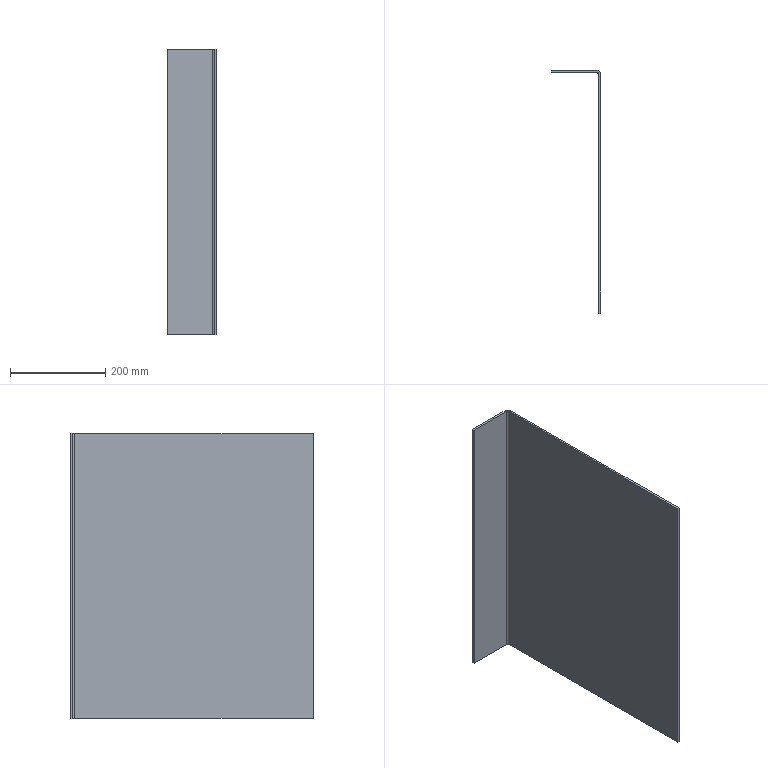Part | STEP file | 03-Side middle pedal | 1 solid | 14 faces | box 104 x 510 x 600 mm | volume 1457819 mm3 | plane 12 | cylinder 2 | commonest cylinder face diameters 8 x1 16 x1
STEP:
#1=CARTESIAN_POINT('',(0.,0.,0.));
#2=DIRECTION('',(0.,0.,1.));
#3=DIRECTION('',(1.,0.,0.));
#4=AXIS2_PLACEMENT_3D('',#1,#2,#3);
#5=CARTESIAN_POINT('',(104.,-8.,600.));
#6=VERTEX_POINT('',#5);
#7=CARTESIAN_POINT('',(100.,-8.,600.));
#8=VERTEX_POINT('',#7);
#9=CARTESIAN_POINT('',(104.,-8.,600.));
#10=DIRECTION('',(-1.,0.,0.));
#11=VECTOR('',#10,1.);
#12=LINE('',#9,#11);
#13=CARTESIAN_POINT('',(104.,-8.,600.));
#14=DIRECTION('',(0.,0.,1.));
#15=DIRECTION('',(1.,0.,0.));
#16=AXIS2_PLACEMENT_3D('',#13,#14,#15);
#17=PLANE('',#16);
#18=CARTESIAN_POINT('',(0.,0.));
#19=DIRECTION('',(-1.,0.));
#20=VECTOR('',#19,1.);
#21=LINE('',#18,#20);
#22=(GEOMETRIC_REPRESENTATION_CONTEXT(2)PARAMETRIC_REPRESENTATION_CONTEXT()REPRESENTATION_CONTEXT('',''));
#23=DEFINITIONAL_REPRESENTATION('',(#21),#22);
#24=PCURVE('',#17,#23);
#25=CARTESIAN_POINT('',(96.,-4.,600.));
#26=DIRECTION('',(0.,0.,1.));
#27=DIRECTION('',(1.,0.,0.));
#28=AXIS2_PLACEMENT_3D('',#25,#26,#27);
#29=PLANE('',#28);
#30=CARTESIAN_POINT('',(8.,-4.));
#31=DIRECTION('',(-1.,0.));
#32=VECTOR('',#31,1.);
#33=LINE('',#30,#32);
#34=(GEOMETRIC_REPRESENTATION_CONTEXT(2)PARAMETRIC_REPRESENTATION_CONTEXT()REPRESENTATION_CONTEXT('',''));
#35=DEFINITIONAL_REPRESENTATION('',(#33),#34);
#36=PCURVE('',#29,#35);
#37=SURFACE_CURVE('',#12,(#24,#36),.PCURVE_S1.);
#38=EDGE_CURVE('',#6,#8,#37,.T.);
#39=ORIENTED_EDGE('',*,*,#38,.F.);
#40=CARTESIAN_POINT('',(96.,0.,600.));
#41=VERTEX_POINT('',#40);
#42=CARTESIAN_POINT('',(96.,-8.,600.));
#43=DIRECTION('',(0.,0.,-1.));
#44=DIRECTION('',(1.,0.,0.));
#45=AXIS2_PLACEMENT_3D('',#42,#43,#44);
#46=CIRCLE('',#45,8.);
#47=CARTESIAN_POINT('',(0.,0.));
#48=CARTESIAN_POINT('',(0.,-13.856));
#49=CARTESIAN_POINT('',(-12.,-6.928));
#50=CARTESIAN_POINT('',(-24.,0.));
#51=CARTESIAN_POINT('',(-12.,6.928));
#52=CARTESIAN_POINT('',(0.,13.856));
#53=CARTESIAN_POINT('',(0.,0.));
#54=(BOUNDED_CURVE()B_SPLINE_CURVE(2,(#47,#48,#49,#50,#51,#52,#53),.UNSPECIFIED.,.T.,.F.)B_SPLINE_CURVE_WITH_KNOTS((1,2,2,2,2,1),(-2.094,0.,2.094,4.189,6.283,8.378),.UNSPECIFIED.)CURVE()GEOMETRIC_REPRESENTATION_ITEM()RATIONAL_B_SPLINE_CURVE((1.,0.5,1.,0.5,1.,0.5,1.))REPRESENTATION_ITEM(''));
#55=(GEOMETRIC_REPRESENTATION_CONTEXT(2)PARAMETRIC_REPRESENTATION_CONTEXT()REPRESENTATION_CONTEXT('',''));
#56=DEFINITIONAL_REPRESENTATION('',(#54),#55);
#57=PCURVE('',#17,#56);
#58=CARTESIAN_POINT('',(96.,-8.,600.));
#59=DIRECTION('',(0.,0.,-1.));
#60=DIRECTION('',(-1.,0.,0.));
#61=AXIS2_PLACEMENT_3D('',#58,#59,#60);
#62=CYLINDRICAL_SURFACE('',#61,8.);
#63=CARTESIAN_POINT('',(-3.142,0.));
#64=DIRECTION('',(1.,0.));
#65=VECTOR('',#64,1.);
#66=LINE('',#63,#65);
#67=(GEOMETRIC_REPRESENTATION_CONTEXT(2)PARAMETRIC_REPRESENTATION_CONTEXT()REPRESENTATION_CONTEXT('',''));
#68=DEFINITIONAL_REPRESENTATION('',(#66),#67);
#69=PCURVE('',#62,#68);
#70=SURFACE_CURVE('',#46,(#57,#69),.PCURVE_S1.);
#71=EDGE_CURVE('',#41,#6,#70,.T.);
#72=ORIENTED_EDGE('',*,*,#71,.F.);
#73=CARTESIAN_POINT('',(96.,-4.,600.));
#74=VERTEX_POINT('',#73);
#75=CARTESIAN_POINT('',(96.,-4.,600.));
#76=DIRECTION('',(0.,1.,0.));
#77=VECTOR('',#76,1.);
#78=LINE('',#75,#77);
#79=CARTESIAN_POINT('',(-8.,4.));
#80=DIRECTION('',(0.,1.));
#81=VECTOR('',#80,1.);
#82=LINE('',#79,#81);
#83=(GEOMETRIC_REPRESENTATION_CONTEXT(2)PARAMETRIC_REPRESENTATION_CONTEXT()REPRESENTATION_CONTEXT('',''));
#84=DEFINITIONAL_REPRESENTATION('',(#82),#83);
#85=PCURVE('',#17,#84);
#86=CARTESIAN_POINT('',(96.,-8.,600.));
#87=DIRECTION('',(0.,0.,1.));
#88=DIRECTION('',(1.,0.,0.));
#89=AXIS2_PLACEMENT_3D('',#86,#87,#88);
#90=PLANE('',#89);
#91=CARTESIAN_POINT('',(0.,4.));
#92=DIRECTION('',(0.,1.));
#93=VECTOR('',#92,1.);
#94=LINE('',#91,#93);
#95=(GEOMETRIC_REPRESENTATION_CONTEXT(2)PARAMETRIC_REPRESENTATION_CONTEXT()REPRESENTATION_CONTEXT('',''));
#96=DEFINITIONAL_REPRESENTATION('',(#94),#95);
#97=PCURVE('',#90,#96);
#98=SURFACE_CURVE('',#78,(#85,#97),.PCURVE_S1.);
#99=EDGE_CURVE('',#74,#41,#98,.T.);
#100=ORIENTED_EDGE('',*,*,#99,.F.);
#101=CARTESIAN_POINT('',(96.,-8.,600.));
#102=DIRECTION('',(0.,0.,-1.));
#103=DIRECTION('',(1.,0.,0.));
#104=AXIS2_PLACEMENT_3D('',#101,#102,#103);
#105=CIRCLE('',#104,4.);
#106=CARTESIAN_POINT('',(-4.,0.));
#107=CARTESIAN_POINT('',(-4.,-6.928));
#108=CARTESIAN_POINT('',(-10.,-3.464));
#109=CARTESIAN_POINT('',(-16.,0.));
#110=CARTESIAN_POINT('',(-10.,3.464));
#111=CARTESIAN_POINT('',(-4.,6.928));
#112=CARTESIAN_POINT('',(-4.,0.));
#113=(BOUNDED_CURVE()B_SPLINE_CURVE(2,(#106,#107,#108,#109,#110,#111,#112),.UNSPECIFIED.,.T.,.F.)B_SPLINE_CURVE_WITH_KNOTS((1,2,2,2,2,1),(-2.094,0.,2.094,4.189,6.283,8.378),.UNSPECIFIED.)CURVE()GEOMETRIC_REPRESENTATION_ITEM()RATIONAL_B_SPLINE_CURVE((1.,0.5,1.,0.5,1.,0.5,1.))REPRESENTATION_ITEM(''));
#114=(GEOMETRIC_REPRESENTATION_CONTEXT(2)PARAMETRIC_REPRESENTATION_CONTEXT()REPRESENTATION_CONTEXT('',''));
#115=DEFINITIONAL_REPRESENTATION('',(#113),#114);
#116=PCURVE('',#17,#115);
#117=CARTESIAN_POINT('',(96.,-8.,600.));
#118=DIRECTION('',(0.,0.,-1.));
#119=DIRECTION('',(-1.,0.,0.));
#120=AXIS2_PLACEMENT_3D('',#117,#118,#119);
#121=CYLINDRICAL_SURFACE('',#120,4.);
#122=CARTESIAN_POINT('',(-3.142,0.));
#123=DIRECTION('',(1.,0.));
#124=VECTOR('',#123,1.);
#125=LINE('',#122,#124);
#126=(GEOMETRIC_REPRESENTATION_CONTEXT(2)PARAMETRIC_REPRESENTATION_CONTEXT()REPRESENTATION_CONTEXT('',''));
#127=DEFINITIONAL_REPRESENTATION('',(#125),#126);
#128=PCURVE('',#121,#127);
#129=SURFACE_CURVE('',#105,(#116,#128),.PCURVE_S1.);
#130=EDGE_CURVE('',#74,#8,#129,.T.);
#131=ORIENTED_EDGE('',*,*,#130,.T.);
#132=EDGE_LOOP('',(#39,#72,#100,#131));
#133=FACE_BOUND('',#132,.T.);
#134=ADVANCED_FACE('',(#133),#17,.T.);
#135=CARTESIAN_POINT('',(104.,-510.,600.));
#136=VERTEX_POINT('',#135);
#137=CARTESIAN_POINT('',(104.,0.,600.));
#138=DIRECTION('',(0.,-1.,0.));
#139=VECTOR('',#138,1.);
#140=LINE('',#137,#139);
#141=CARTESIAN_POINT('',(8.,4.));
#142=DIRECTION('',(0.,-1.));
#143=VECTOR('',#142,1.);
#144=LINE('',#141,#143);
#145=(GEOMETRIC_REPRESENTATION_CONTEXT(2)PARAMETRIC_REPRESENTATION_CONTEXT()REPRESENTATION_CONTEXT('',''));
#146=DEFINITIONAL_REPRESENTATION('',(#144),#145);
#147=PCURVE('',#29,#146);
#148=CARTESIAN_POINT('',(104.,0.,600.));
#149=DIRECTION('',(1.,0.,0.));
#150=DIRECTION('',(0.,1.,0.));
#151=AXIS2_PLACEMENT_3D('',#148,#149,#150);
#152=PLANE('',#151);
#153=CARTESIAN_POINT('',(0.,0.));
#154=DIRECTION('',(-1.,0.));
#155=VECTOR('',#154,1.);
#156=LINE('',#153,#155);
#157=(GEOMETRIC_REPRESENTATION_CONTEXT(2)PARAMETRIC_REPRESENTATION_CONTEXT()REPRESENTATION_CONTEXT('',''));
#158=DEFINITIONAL_REPRESENTATION('',(#156),#157);
#159=PCURVE('',#152,#158);
#160=SURFACE_CURVE('',#140,(#147,#159),.PCURVE_S1.);
#161=EDGE_CURVE('',#6,#136,#160,.T.);
#162=ORIENTED_EDGE('',*,*,#161,.F.);
#163=ORIENTED_EDGE('',*,*,#38,.T.);
#164=CARTESIAN_POINT('',(100.,-510.,600.));
#165=VERTEX_POINT('',#164);
#166=CARTESIAN_POINT('',(100.,0.,600.));
#167=DIRECTION('',(0.,-1.,0.));
#168=VECTOR('',#167,1.);
#169=LINE('',#166,#168);
#170=CARTESIAN_POINT('',(4.,4.));
#171=DIRECTION('',(0.,-1.));
#172=VECTOR('',#171,1.);
#173=LINE('',#170,#172);
#174=(GEOMETRIC_REPRESENTATION_CONTEXT(2)PARAMETRIC_REPRESENTATION_CONTEXT()REPRESENTATION_CONTEXT('',''));
#175=DEFINITIONAL_REPRESENTATION('',(#173),#174);
#176=PCURVE('',#29,#175);
#177=CARTESIAN_POINT('',(100.,0.,600.));
#178=DIRECTION('',(1.,0.,0.));
#179=DIRECTION('',(0.,1.,0.));
#180=AXIS2_PLACEMENT_3D('',#177,#178,#179);
#181=PLANE('',#180);
#182=CARTESIAN_POINT('',(0.,0.));
#183=DIRECTION('',(-1.,0.));
#184=VECTOR('',#183,1.);
#185=LINE('',#182,#184);
#186=(GEOMETRIC_REPRESENTATION_CONTEXT(2)PARAMETRIC_REPRESENTATION_CONTEXT()REPRESENTATION_CONTEXT('',''));
#187=DEFINITIONAL_REPRESENTATION('',(#185),#186);
#188=PCURVE('',#181,#187);
#189=SURFACE_CURVE('',#169,(#176,#188),.PCURVE_S1.);
#190=EDGE_CURVE('',#8,#165,#189,.T.);
#191=ORIENTED_EDGE('',*,*,#190,.T.);
#192=CARTESIAN_POINT('',(104.,-510.,600.));
#193=DIRECTION('',(-1.,0.,0.));
#194=VECTOR('',#193,1.);
#195=LINE('',#192,#194);
#196=CARTESIAN_POINT('',(8.,-506.));
#197=DIRECTION('',(-1.,0.));
#198=VECTOR('',#197,1.);
#199=LINE('',#196,#198);
#200=(GEOMETRIC_REPRESENTATION_CONTEXT(2)PARAMETRIC_REPRESENTATION_CONTEXT()REPRESENTATION_CONTEXT('',''));
#201=DEFINITIONAL_REPRESENTATION('',(#199),#200);
#202=PCURVE('',#29,#201);
#203=CARTESIAN_POINT('',(104.,-510.,600.));
#204=DIRECTION('',(0.,-1.,0.));
#205=DIRECTION('',(0.,0.,-1.));
#206=AXIS2_PLACEMENT_3D('',#203,#204,#205);
#207=PLANE('',#206);
#208=CARTESIAN_POINT('',(0.,0.));
#209=DIRECTION('',(0.,-1.));
#210=VECTOR('',#209,1.);
#211=LINE('',#208,#210);
#212=(GEOMETRIC_REPRESENTATION_CONTEXT(2)PARAMETRIC_REPRESENTATION_CONTEXT()REPRESENTATION_CONTEXT('',''));
#213=DEFINITIONAL_REPRESENTATION('',(#211),#212);
#214=PCURVE('',#207,#213);
#215=SURFACE_CURVE('',#195,(#202,#214),.PCURVE_S1.);
#216=EDGE_CURVE('',#136,#165,#215,.T.);
#217=ORIENTED_EDGE('',*,*,#216,.F.);
#218=EDGE_LOOP('',(#162,#163,#191,#217));
#219=FACE_BOUND('',#218,.T.);
#220=ADVANCED_FACE('',(#219),#29,.T.);
#221=CARTESIAN_POINT('',(96.,0.,0.));
#222=VERTEX_POINT('',#221);
#223=CARTESIAN_POINT('',(96.,-4.,0.));
#224=VERTEX_POINT('',#223);
#225=CARTESIAN_POINT('',(96.,0.,0.));
#226=DIRECTION('',(0.,-1.,0.));
#227=VECTOR('',#226,1.);
#228=LINE('',#225,#227);
#229=CARTESIAN_POINT('',(96.,0.,0.));
#230=DIRECTION('',(0.,0.,-1.));
#231=DIRECTION('',(-1.,0.,0.));
#232=AXIS2_PLACEMENT_3D('',#229,#230,#231);
#233=PLANE('',#232);
#234=CARTESIAN_POINT('',(0.,0.));
#235=DIRECTION('',(0.,-1.));
#236=VECTOR('',#235,1.);
#237=LINE('',#234,#236);
#238=(GEOMETRIC_REPRESENTATION_CONTEXT(2)PARAMETRIC_REPRESENTATION_CONTEXT()REPRESENTATION_CONTEXT('',''));
#239=DEFINITIONAL_REPRESENTATION('',(#237),#238);
#240=PCURVE('',#233,#239);
#241=CARTESIAN_POINT('',(100.,-8.,0.));
#242=DIRECTION('',(0.,0.,-1.));
#243=DIRECTION('',(-1.,0.,0.));
#244=AXIS2_PLACEMENT_3D('',#241,#242,#243);
#245=PLANE('',#244);
#246=CARTESIAN_POINT('',(4.,8.));
#247=DIRECTION('',(0.,-1.));
#248=VECTOR('',#247,1.);
#249=LINE('',#246,#248);
#250=(GEOMETRIC_REPRESENTATION_CONTEXT(2)PARAMETRIC_REPRESENTATION_CONTEXT()REPRESENTATION_CONTEXT('',''));
#251=DEFINITIONAL_REPRESENTATION('',(#249),#250);
#252=PCURVE('',#245,#251);
#253=SURFACE_CURVE('',#228,(#240,#252),.PCURVE_S1.);
#254=EDGE_CURVE('',#222,#224,#253,.T.);
#255=ORIENTED_EDGE('',*,*,#254,.F.);
#256=CARTESIAN_POINT('',(104.,-8.,0.));
#257=VERTEX_POINT('',#256);
#258=CARTESIAN_POINT('',(96.,-8.,0.));
#259=DIRECTION('',(0.,0.,-1.));
#260=DIRECTION('',(1.,0.,0.));
#261=AXIS2_PLACEMENT_3D('',#258,#259,#260);
#262=CIRCLE('',#261,8.);
#263=CARTESIAN_POINT('',(0.,-8.));
#264=DIRECTION('',(-1.,0.));
#265=AXIS2_PLACEMENT_2D('',#263,#264);
#266=CIRCLE('',#265,8.);
#267=(GEOMETRIC_REPRESENTATION_CONTEXT(2)PARAMETRIC_REPRESENTATION_CONTEXT()REPRESENTATION_CONTEXT('',''));
#268=DEFINITIONAL_REPRESENTATION('',(#266),#267);
#269=PCURVE('',#233,#268);
#270=CARTESIAN_POINT('',(-3.142,600.));
#271=DIRECTION('',(1.,0.));
#272=VECTOR('',#271,1.);
#273=LINE('',#270,#272);
#274=(GEOMETRIC_REPRESENTATION_CONTEXT(2)PARAMETRIC_REPRESENTATION_CONTEXT()REPRESENTATION_CONTEXT('',''));
#275=DEFINITIONAL_REPRESENTATION('',(#273),#274);
#276=PCURVE('',#62,#275);
#277=SURFACE_CURVE('',#262,(#269,#276),.PCURVE_S1.);
#278=EDGE_CURVE('',#222,#257,#277,.T.);
#279=ORIENTED_EDGE('',*,*,#278,.T.);
#280=CARTESIAN_POINT('',(100.,-8.,0.));
#281=VERTEX_POINT('',#280);
#282=CARTESIAN_POINT('',(100.,-8.,0.));
#283=DIRECTION('',(1.,0.,0.));
#284=VECTOR('',#283,1.);
#285=LINE('',#282,#284);
#286=CARTESIAN_POINT('',(-4.,-8.));
#287=DIRECTION('',(-1.,0.));
#288=VECTOR('',#287,1.);
#289=LINE('',#286,#288);
#290=(GEOMETRIC_REPRESENTATION_CONTEXT(2)PARAMETRIC_REPRESENTATION_CONTEXT()REPRESENTATION_CONTEXT('',''));
#291=DEFINITIONAL_REPRESENTATION('',(#289),#290);
#292=PCURVE('',#233,#291);
#293=CARTESIAN_POINT('',(96.,-8.,0.));
#294=DIRECTION('',(0.,0.,1.));
#295=DIRECTION('',(1.,0.,0.));
#296=AXIS2_PLACEMENT_3D('',#293,#294,#295);
#297=PLANE('',#296);
#298=CARTESIAN_POINT('',(4.,0.));
#299=DIRECTION('',(1.,0.));
#300=VECTOR('',#299,1.);
#301=LINE('',#298,#300);
#302=(GEOMETRIC_REPRESENTATION_CONTEXT(2)PARAMETRIC_REPRESENTATION_CONTEXT()REPRESENTATION_CONTEXT('',''));
#303=DEFINITIONAL_REPRESENTATION('',(#301),#302);
#304=PCURVE('',#297,#303);
#305=SURFACE_CURVE('',#285,(#292,#304),.PCURVE_S1.);
#306=EDGE_CURVE('',#281,#257,#305,.T.);
#307=ORIENTED_EDGE('',*,*,#306,.F.);
#308=CARTESIAN_POINT('',(96.,-8.,0.));
#309=DIRECTION('',(0.,0.,-1.));
#310=DIRECTION('',(1.,0.,0.));
#311=AXIS2_PLACEMENT_3D('',#308,#309,#310);
#312=CIRCLE('',#311,4.);
#313=CARTESIAN_POINT('',(0.,-8.));
#314=DIRECTION('',(-1.,0.));
#315=AXIS2_PLACEMENT_2D('',#313,#314);
#316=CIRCLE('',#315,4.);
#317=(GEOMETRIC_REPRESENTATION_CONTEXT(2)PARAMETRIC_REPRESENTATION_CONTEXT()REPRESENTATION_CONTEXT('',''));
#318=DEFINITIONAL_REPRESENTATION('',(#316),#317);
#319=PCURVE('',#233,#318);
#320=CARTESIAN_POINT('',(-3.142,600.));
#321=DIRECTION('',(1.,0.));
#322=VECTOR('',#321,1.);
#323=LINE('',#320,#322);
#324=(GEOMETRIC_REPRESENTATION_CONTEXT(2)PARAMETRIC_REPRESENTATION_CONTEXT()REPRESENTATION_CONTEXT('',''));
#325=DEFINITIONAL_REPRESENTATION('',(#323),#324);
#326=PCURVE('',#121,#325);
#327=SURFACE_CURVE('',#312,(#319,#326),.PCURVE_S1.);
#328=EDGE_CURVE('',#224,#281,#327,.T.);
#329=ORIENTED_EDGE('',*,*,#328,.F.);
#330=EDGE_LOOP('',(#255,#279,#307,#329));
#331=FACE_BOUND('',#330,.T.);
#332=ADVANCED_FACE('',(#331),#233,.T.);
#333=CARTESIAN_POINT('',(0.,0.,0.));
#334=VERTEX_POINT('',#333);
#335=CARTESIAN_POINT('',(0.,0.,0.));
#336=DIRECTION('',(1.,0.,0.));
#337=VECTOR('',#336,1.);
#338=LINE('',#335,#337);
#339=CARTESIAN_POINT('',(100.,8.));
#340=DIRECTION('',(-1.,0.));
#341=VECTOR('',#340,1.);
#342=LINE('',#339,#341);
#343=(GEOMETRIC_REPRESENTATION_CONTEXT(2)PARAMETRIC_REPRESENTATION_CONTEXT()REPRESENTATION_CONTEXT('',''));
#344=DEFINITIONAL_REPRESENTATION('',(#342),#343);
#345=PCURVE('',#245,#344);
#346=CARTESIAN_POINT('',(0.,0.,600.));
#347=DIRECTION('',(0.,1.,0.));
#348=DIRECTION('',(0.,0.,1.));
#349=AXIS2_PLACEMENT_3D('',#346,#347,#348);
#350=PLANE('',#349);
#351=CARTESIAN_POINT('',(-600.,0.));
#352=DIRECTION('',(0.,1.));
#353=VECTOR('',#352,1.);
#354=LINE('',#351,#353);
#355=(GEOMETRIC_REPRESENTATION_CONTEXT(2)PARAMETRIC_REPRESENTATION_CONTEXT()REPRESENTATION_CONTEXT('',''));
#356=DEFINITIONAL_REPRESENTATION('',(#354),#355);
#357=PCURVE('',#350,#356);
#358=SURFACE_CURVE('',#338,(#345,#357),.PCURVE_S1.);
#359=EDGE_CURVE('',#334,#222,#358,.T.);
#360=ORIENTED_EDGE('',*,*,#359,.T.);
#361=ORIENTED_EDGE('',*,*,#254,.T.);
#362=CARTESIAN_POINT('',(0.,-4.,0.));
#363=VERTEX_POINT('',#362);
#364=CARTESIAN_POINT('',(0.,-4.,0.));
#365=DIRECTION('',(1.,0.,0.));
#366=VECTOR('',#365,1.);
#367=LINE('',#364,#366);
#368=CARTESIAN_POINT('',(100.,4.));
#369=DIRECTION('',(-1.,0.));
#370=VECTOR('',#369,1.);
#371=LINE('',#368,#370);
#372=(GEOMETRIC_REPRESENTATION_CONTEXT(2)PARAMETRIC_REPRESENTATION_CONTEXT()REPRESENTATION_CONTEXT('',''));
#373=DEFINITIONAL_REPRESENTATION('',(#371),#372);
#374=PCURVE('',#245,#373);
#375=CARTESIAN_POINT('',(0.,-4.,600.));
#376=DIRECTION('',(0.,1.,0.));
#377=DIRECTION('',(0.,0.,1.));
#378=AXIS2_PLACEMENT_3D('',#375,#376,#377);
#379=PLANE('',#378);
#380=CARTESIAN_POINT('',(-600.,0.));
#381=DIRECTION('',(0.,1.));
#382=VECTOR('',#381,1.);
#383=LINE('',#380,#382);
#384=(GEOMETRIC_REPRESENTATION_CONTEXT(2)PARAMETRIC_REPRESENTATION_CONTEXT()REPRESENTATION_CONTEXT('',''));
#385=DEFINITIONAL_REPRESENTATION('',(#383),#384);
#386=PCURVE('',#379,#385);
#387=SURFACE_CURVE('',#367,(#374,#386),.PCURVE_S1.);
#388=EDGE_CURVE('',#363,#224,#387,.T.);
#389=ORIENTED_EDGE('',*,*,#388,.F.);
#390=CARTESIAN_POINT('',(0.,-4.,0.));
#391=DIRECTION('',(0.,1.,0.));
#392=VECTOR('',#391,1.);
#393=LINE('',#390,#392);
#394=CARTESIAN_POINT('',(100.,4.));
#395=DIRECTION('',(0.,1.));
#396=VECTOR('',#395,1.);
#397=LINE('',#394,#396);
#398=(GEOMETRIC_REPRESENTATION_CONTEXT(2)PARAMETRIC_REPRESENTATION_CONTEXT()REPRESENTATION_CONTEXT('',''));
#399=DEFINITIONAL_REPRESENTATION('',(#397),#398);
#400=PCURVE('',#245,#399);
#401=CARTESIAN_POINT('',(0.,-4.,600.));
#402=DIRECTION('',(-1.,0.,0.));
#403=DIRECTION('',(0.,0.,1.));
#404=AXIS2_PLACEMENT_3D('',#401,#402,#403);
#405=PLANE('',#404);
#406=CARTESIAN_POINT('',(-600.,0.));
#407=DIRECTION('',(0.,1.));
#408=VECTOR('',#407,1.);
#409=LINE('',#406,#408);
#410=(GEOMETRIC_REPRESENTATION_CONTEXT(2)PARAMETRIC_REPRESENTATION_CONTEXT()REPRESENTATION_CONTEXT('',''));
#411=DEFINITIONAL_REPRESENTATION('',(#409),#410);
#412=PCURVE('',#405,#411);
#413=SURFACE_CURVE('',#393,(#400,#412),.PCURVE_S1.);
#414=EDGE_CURVE('',#363,#334,#413,.T.);
#415=ORIENTED_EDGE('',*,*,#414,.T.);
#416=EDGE_LOOP('',(#360,#361,#389,#415));
#417=FACE_BOUND('',#416,.T.);
#418=ADVANCED_FACE('',(#417),#245,.T.);
#419=CARTESIAN_POINT('',(100.,-510.,0.));
#420=VERTEX_POINT('',#419);
#421=CARTESIAN_POINT('',(100.,0.,0.));
#422=DIRECTION('',(0.,-1.,0.));
#423=VECTOR('',#422,1.);
#424=LINE('',#421,#423);
#425=CARTESIAN_POINT('',(0.,-600.));
#426=DIRECTION('',(-1.,0.));
#427=VECTOR('',#426,1.);
#428=LINE('',#425,#427);
#429=(GEOMETRIC_REPRESENTATION_CONTEXT(2)PARAMETRIC_REPRESENTATION_CONTEXT()REPRESENTATION_CONTEXT('',''));
#430=DEFINITIONAL_REPRESENTATION('',(#428),#429);
#431=PCURVE('',#181,#430);
#432=CARTESIAN_POINT('',(4.,8.));
#433=DIRECTION('',(0.,-1.));
#434=VECTOR('',#433,1.);
#435=LINE('',#432,#434);
#436=(GEOMETRIC_REPRESENTATION_CONTEXT(2)PARAMETRIC_REPRESENTATION_CONTEXT()REPRESENTATION_CONTEXT('',''));
#437=DEFINITIONAL_REPRESENTATION('',(#435),#436);
#438=PCURVE('',#297,#437);
#439=SURFACE_CURVE('',#424,(#431,#438),.PCURVE_S1.);
#440=EDGE_CURVE('',#281,#420,#439,.T.);
#441=ORIENTED_EDGE('',*,*,#440,.T.);
#442=CARTESIAN_POINT('',(100.,-510.,600.));
#443=DIRECTION('',(0.,0.,-1.));
#444=VECTOR('',#443,1.);
#445=LINE('',#442,#444);
#446=CARTESIAN_POINT('',(-510.,0.));
#447=DIRECTION('',(0.,-1.));
#448=VECTOR('',#447,1.);
#449=LINE('',#446,#448);
#450=(GEOMETRIC_REPRESENTATION_CONTEXT(2)PARAMETRIC_REPRESENTATION_CONTEXT()REPRESENTATION_CONTEXT('',''));
#451=DEFINITIONAL_REPRESENTATION('',(#449),#450);
#452=PCURVE('',#181,#451);
#453=CARTESIAN_POINT('',(0.,-4.));
#454=DIRECTION('',(1.,0.));
#455=VECTOR('',#454,1.);
#456=LINE('',#453,#455);
#457=(GEOMETRIC_REPRESENTATION_CONTEXT(2)PARAMETRIC_REPRESENTATION_CONTEXT()REPRESENTATION_CONTEXT('',''));
#458=DEFINITIONAL_REPRESENTATION('',(#456),#457);
#459=PCURVE('',#207,#458);
#460=SURFACE_CURVE('',#445,(#452,#459),.PCURVE_S1.);
#461=EDGE_CURVE('',#165,#420,#460,.T.);
#462=ORIENTED_EDGE('',*,*,#461,.F.);
#463=ORIENTED_EDGE('',*,*,#190,.F.);
#464=CARTESIAN_POINT('',(100.,-8.,600.));
#465=DIRECTION('',(0.,0.,-1.));
#466=VECTOR('',#465,1.);
#467=LINE('',#464,#466);
#468=CARTESIAN_POINT('',(-8.,0.));
#469=DIRECTION('',(0.,-1.));
#470=VECTOR('',#469,1.);
#471=LINE('',#468,#470);
#472=(GEOMETRIC_REPRESENTATION_CONTEXT(2)PARAMETRIC_REPRESENTATION_CONTEXT()REPRESENTATION_CONTEXT('',''));
#473=DEFINITIONAL_REPRESENTATION('',(#471),#472);
#474=PCURVE('',#181,#473);
#475=CARTESIAN_POINT('',(3.142,0.));
#476=DIRECTION('',(0.,1.));
#477=VECTOR('',#476,1.);
#478=LINE('',#475,#477);
#479=(GEOMETRIC_REPRESENTATION_CONTEXT(2)PARAMETRIC_REPRESENTATION_CONTEXT()REPRESENTATION_CONTEXT('',''));
#480=DEFINITIONAL_REPRESENTATION('',(#478),#479);
#481=PCURVE('',#121,#480);
#482=SURFACE_CURVE('',#467,(#474,#481),.PCURVE_S1.);
#483=EDGE_CURVE('',#8,#281,#482,.T.);
#484=ORIENTED_EDGE('',*,*,#483,.T.);
#485=EDGE_LOOP('',(#441,#462,#463,#484));
#486=FACE_BOUND('',#485,.T.);
#487=ADVANCED_FACE('',(#486),#181,.F.);
#488=CARTESIAN_POINT('',(104.,-510.,0.));
#489=VERTEX_POINT('',#488);
#490=CARTESIAN_POINT('',(104.,-510.,0.));
#491=DIRECTION('',(-1.,0.,0.));
#492=VECTOR('',#491,1.);
#493=LINE('',#490,#492);
#494=CARTESIAN_POINT('',(600.,0.));
#495=DIRECTION('',(0.,-1.));
#496=VECTOR('',#495,1.);
#497=LINE('',#494,#496);
#498=(GEOMETRIC_REPRESENTATION_CONTEXT(2)PARAMETRIC_REPRESENTATION_CONTEXT()REPRESENTATION_CONTEXT('',''));
#499=DEFINITIONAL_REPRESENTATION('',(#497),#498);
#500=PCURVE('',#207,#499);
#501=CARTESIAN_POINT('',(8.,-502.));
#502=DIRECTION('',(-1.,0.));
#503=VECTOR('',#502,1.);
#504=LINE('',#501,#503);
#505=(GEOMETRIC_REPRESENTATION_CONTEXT(2)PARAMETRIC_REPRESENTATION_CONTEXT()REPRESENTATION_CONTEXT('',''));
#506=DEFINITIONAL_REPRESENTATION('',(#504),#505);
#507=PCURVE('',#297,#506);
#508=SURFACE_CURVE('',#493,(#500,#507),.PCURVE_S1.);
#509=EDGE_CURVE('',#489,#420,#508,.T.);
#510=ORIENTED_EDGE('',*,*,#509,.F.);
#511=CARTESIAN_POINT('',(104.,-510.,600.));
#512=DIRECTION('',(0.,0.,-1.));
#513=VECTOR('',#512,1.);
#514=LINE('',#511,#513);
#515=CARTESIAN_POINT('',(0.,0.));
#516=DIRECTION('',(1.,0.));
#517=VECTOR('',#516,1.);
#518=LINE('',#515,#517);
#519=(GEOMETRIC_REPRESENTATION_CONTEXT(2)PARAMETRIC_REPRESENTATION_CONTEXT()REPRESENTATION_CONTEXT('',''));
#520=DEFINITIONAL_REPRESENTATION('',(#518),#519);
#521=PCURVE('',#207,#520);
#522=CARTESIAN_POINT('',(-510.,0.));
#523=DIRECTION('',(0.,-1.));
#524=VECTOR('',#523,1.);
#525=LINE('',#522,#524);
#526=(GEOMETRIC_REPRESENTATION_CONTEXT(2)PARAMETRIC_REPRESENTATION_CONTEXT()REPRESENTATION_CONTEXT('',''));
#527=DEFINITIONAL_REPRESENTATION('',(#525),#526);
#528=PCURVE('',#152,#527);
#529=SURFACE_CURVE('',#514,(#521,#528),.PCURVE_S1.);
#530=EDGE_CURVE('',#136,#489,#529,.T.);
#531=ORIENTED_EDGE('',*,*,#530,.F.);
#532=ORIENTED_EDGE('',*,*,#216,.T.);
#533=ORIENTED_EDGE('',*,*,#461,.T.);
#534=EDGE_LOOP('',(#510,#531,#532,#533));
#535=FACE_BOUND('',#534,.T.);
#536=ADVANCED_FACE('',(#535),#207,.T.);
#537=CARTESIAN_POINT('',(104.,0.,0.));
#538=DIRECTION('',(0.,-1.,0.));
#539=VECTOR('',#538,1.);
#540=LINE('',#537,#539);
#541=CARTESIAN_POINT('',(0.,-600.));
#542=DIRECTION('',(-1.,0.));
#543=VECTOR('',#542,1.);
#544=LINE('',#541,#543);
#545=(GEOMETRIC_REPRESENTATION_CONTEXT(2)PARAMETRIC_REPRESENTATION_CONTEXT()REPRESENTATION_CONTEXT('',''));
#546=DEFINITIONAL_REPRESENTATION('',(#544),#545);
#547=PCURVE('',#152,#546);
#548=CARTESIAN_POINT('',(8.,8.));
#549=DIRECTION('',(0.,-1.));
#550=VECTOR('',#549,1.);
#551=LINE('',#548,#550);
#552=(GEOMETRIC_REPRESENTATION_CONTEXT(2)PARAMETRIC_REPRESENTATION_CONTEXT()REPRESENTATION_CONTEXT('',''));
#553=DEFINITIONAL_REPRESENTATION('',(#551),#552);
#554=PCURVE('',#297,#553);
#555=SURFACE_CURVE('',#540,(#547,#554),.PCURVE_S1.);
#556=EDGE_CURVE('',#257,#489,#555,.T.);
#557=ORIENTED_EDGE('',*,*,#556,.F.);
#558=CARTESIAN_POINT('',(104.,-8.,600.));
#559=DIRECTION('',(0.,0.,-1.));
#560=VECTOR('',#559,1.);
#561=LINE('',#558,#560);
#562=CARTESIAN_POINT('',(-8.,0.));
#563=DIRECTION('',(0.,-1.));
#564=VECTOR('',#563,1.);
#565=LINE('',#562,#564);
#566=(GEOMETRIC_REPRESENTATION_CONTEXT(2)PARAMETRIC_REPRESENTATION_CONTEXT()REPRESENTATION_CONTEXT('',''));
#567=DEFINITIONAL_REPRESENTATION('',(#565),#566);
#568=PCURVE('',#152,#567);
#569=CARTESIAN_POINT('',(3.142,0.));
#570=DIRECTION('',(0.,1.));
#571=VECTOR('',#570,1.);
#572=LINE('',#569,#571);
#573=(GEOMETRIC_REPRESENTATION_CONTEXT(2)PARAMETRIC_REPRESENTATION_CONTEXT()REPRESENTATION_CONTEXT('',''));
#574=DEFINITIONAL_REPRESENTATION('',(#572),#573);
#575=PCURVE('',#62,#574);
#576=SURFACE_CURVE('',#561,(#568,#575),.PCURVE_S1.);
#577=EDGE_CURVE('',#6,#257,#576,.T.);
#578=ORIENTED_EDGE('',*,*,#577,.F.);
#579=ORIENTED_EDGE('',*,*,#161,.T.);
#580=ORIENTED_EDGE('',*,*,#530,.T.);
#581=EDGE_LOOP('',(#557,#578,#579,#580));
#582=FACE_BOUND('',#581,.T.);
#583=ADVANCED_FACE('',(#582),#152,.T.);
#584=ORIENTED_EDGE('',*,*,#278,.F.);
#585=CARTESIAN_POINT('',(96.,0.,600.));
#586=DIRECTION('',(0.,0.,-1.));
#587=VECTOR('',#586,1.);
#588=LINE('',#585,#587);
#589=CARTESIAN_POINT('',(1.571,0.));
#590=DIRECTION('',(0.,1.));
#591=VECTOR('',#590,1.);
#592=LINE('',#589,#591);
#593=(GEOMETRIC_REPRESENTATION_CONTEXT(2)PARAMETRIC_REPRESENTATION_CONTEXT()REPRESENTATION_CONTEXT('',''));
#594=DEFINITIONAL_REPRESENTATION('',(#592),#593);
#595=PCURVE('',#62,#594);
#596=CARTESIAN_POINT('',(0.,96.));
#597=DIRECTION('',(-1.,0.));
#598=VECTOR('',#597,1.);
#599=LINE('',#596,#598);
#600=(GEOMETRIC_REPRESENTATION_CONTEXT(2)PARAMETRIC_REPRESENTATION_CONTEXT()REPRESENTATION_CONTEXT('',''));
#601=DEFINITIONAL_REPRESENTATION('',(#599),#600);
#602=PCURVE('',#350,#601);
#603=SURFACE_CURVE('',#588,(#595,#602),.PCURVE_S1.);
#604=EDGE_CURVE('',#41,#222,#603,.T.);
#605=ORIENTED_EDGE('',*,*,#604,.F.);
#606=ORIENTED_EDGE('',*,*,#71,.T.);
#607=ORIENTED_EDGE('',*,*,#577,.T.);
#608=EDGE_LOOP('',(#584,#605,#606,#607));
#609=FACE_BOUND('',#608,.T.);
#610=ADVANCED_FACE('',(#609),#62,.T.);
#611=ORIENTED_EDGE('',*,*,#359,.F.);
#612=CARTESIAN_POINT('',(0.,0.,600.));
#613=VERTEX_POINT('',#612);
#614=CARTESIAN_POINT('',(0.,0.,600.));
#615=DIRECTION('',(0.,0.,-1.));
#616=VECTOR('',#615,1.);
#617=LINE('',#614,#616);
#618=CARTESIAN_POINT('',(0.,0.));
#619=DIRECTION('',(-1.,0.));
#620=VECTOR('',#619,1.);
#621=LINE('',#618,#620);
#622=(GEOMETRIC_REPRESENTATION_CONTEXT(2)PARAMETRIC_REPRESENTATION_CONTEXT()REPRESENTATION_CONTEXT('',''));
#623=DEFINITIONAL_REPRESENTATION('',(#621),#622);
#624=PCURVE('',#350,#623);
#625=CARTESIAN_POINT('',(0.,4.));
#626=DIRECTION('',(-1.,0.));
#627=VECTOR('',#626,1.);
#628=LINE('',#625,#627);
#629=(GEOMETRIC_REPRESENTATION_CONTEXT(2)PARAMETRIC_REPRESENTATION_CONTEXT()REPRESENTATION_CONTEXT('',''));
#630=DEFINITIONAL_REPRESENTATION('',(#628),#629);
#631=PCURVE('',#405,#630);
#632=SURFACE_CURVE('',#617,(#624,#631),.PCURVE_S1.);
#633=EDGE_CURVE('',#613,#334,#632,.T.);
#634=ORIENTED_EDGE('',*,*,#633,.F.);
#635=CARTESIAN_POINT('',(0.,0.,600.));
#636=DIRECTION('',(1.,0.,0.));
#637=VECTOR('',#636,1.);
#638=LINE('',#635,#637);
#639=CARTESIAN_POINT('',(0.,0.));
#640=DIRECTION('',(0.,1.));
#641=VECTOR('',#640,1.);
#642=LINE('',#639,#641);
#643=(GEOMETRIC_REPRESENTATION_CONTEXT(2)PARAMETRIC_REPRESENTATION_CONTEXT()REPRESENTATION_CONTEXT('',''));
#644=DEFINITIONAL_REPRESENTATION('',(#642),#643);
#645=PCURVE('',#350,#644);
#646=CARTESIAN_POINT('',(-96.,8.));
#647=DIRECTION('',(1.,0.));
#648=VECTOR('',#647,1.);
#649=LINE('',#646,#648);
#650=(GEOMETRIC_REPRESENTATION_CONTEXT(2)PARAMETRIC_REPRESENTATION_CONTEXT()REPRESENTATION_CONTEXT('',''));
#651=DEFINITIONAL_REPRESENTATION('',(#649),#650);
#652=PCURVE('',#90,#651);
#653=SURFACE_CURVE('',#638,(#645,#652),.PCURVE_S1.);
#654=EDGE_CURVE('',#613,#41,#653,.T.);
#655=ORIENTED_EDGE('',*,*,#654,.T.);
#656=ORIENTED_EDGE('',*,*,#604,.T.);
#657=EDGE_LOOP('',(#611,#634,#655,#656));
#658=FACE_BOUND('',#657,.T.);
#659=ADVANCED_FACE('',(#658),#350,.T.);
#660=ORIENTED_EDGE('',*,*,#414,.F.);
#661=CARTESIAN_POINT('',(0.,-4.,600.));
#662=VERTEX_POINT('',#661);
#663=CARTESIAN_POINT('',(0.,-4.,600.));
#664=DIRECTION('',(0.,0.,-1.));
#665=VECTOR('',#664,1.);
#666=LINE('',#663,#665);
#667=CARTESIAN_POINT('',(0.,0.));
#668=DIRECTION('',(-1.,0.));
#669=VECTOR('',#668,1.);
#670=LINE('',#667,#669);
#671=(GEOMETRIC_REPRESENTATION_CONTEXT(2)PARAMETRIC_REPRESENTATION_CONTEXT()REPRESENTATION_CONTEXT('',''));
#672=DEFINITIONAL_REPRESENTATION('',(#670),#671);
#673=PCURVE('',#405,#672);
#674=CARTESIAN_POINT('',(0.,0.));
#675=DIRECTION('',(-1.,0.));
#676=VECTOR('',#675,1.);
#677=LINE('',#674,#676);
#678=(GEOMETRIC_REPRESENTATION_CONTEXT(2)PARAMETRIC_REPRESENTATION_CONTEXT()REPRESENTATION_CONTEXT('',''));
#679=DEFINITIONAL_REPRESENTATION('',(#677),#678);
#680=PCURVE('',#379,#679);
#681=SURFACE_CURVE('',#666,(#673,#680),.PCURVE_S1.);
#682=EDGE_CURVE('',#662,#363,#681,.T.);
#683=ORIENTED_EDGE('',*,*,#682,.F.);
#684=CARTESIAN_POINT('',(0.,-4.,600.));
#685=DIRECTION('',(0.,1.,0.));
#686=VECTOR('',#685,1.);
#687=LINE('',#684,#686);
#688=CARTESIAN_POINT('',(0.,0.));
#689=DIRECTION('',(0.,1.));
#690=VECTOR('',#689,1.);
#691=LINE('',#688,#690);
#692=(GEOMETRIC_REPRESENTATION_CONTEXT(2)PARAMETRIC_REPRESENTATION_CONTEXT()REPRESENTATION_CONTEXT('',''));
#693=DEFINITIONAL_REPRESENTATION('',(#691),#692);
#694=PCURVE('',#405,#693);
#695=CARTESIAN_POINT('',(-96.,4.));
#696=DIRECTION('',(0.,1.));
#697=VECTOR('',#696,1.);
#698=LINE('',#695,#697);
#699=(GEOMETRIC_REPRESENTATION_CONTEXT(2)PARAMETRIC_REPRESENTATION_CONTEXT()REPRESENTATION_CONTEXT('',''));
#700=DEFINITIONAL_REPRESENTATION('',(#698),#699);
#701=PCURVE('',#90,#700);
#702=SURFACE_CURVE('',#687,(#694,#701),.PCURVE_S1.);
#703=EDGE_CURVE('',#662,#613,#702,.T.);
#704=ORIENTED_EDGE('',*,*,#703,.T.);
#705=ORIENTED_EDGE('',*,*,#633,.T.);
#706=EDGE_LOOP('',(#660,#683,#704,#705));
#707=FACE_BOUND('',#706,.T.);
#708=ADVANCED_FACE('',(#707),#405,.T.);
#709=ORIENTED_EDGE('',*,*,#388,.T.);
#710=CARTESIAN_POINT('',(96.,-4.,600.));
#711=DIRECTION('',(0.,0.,-1.));
#712=VECTOR('',#711,1.);
#713=LINE('',#710,#712);
#714=CARTESIAN_POINT('',(0.,96.));
#715=DIRECTION('',(-1.,0.));
#716=VECTOR('',#715,1.);
#717=LINE('',#714,#716);
#718=(GEOMETRIC_REPRESENTATION_CONTEXT(2)PARAMETRIC_REPRESENTATION_CONTEXT()REPRESENTATION_CONTEXT('',''));
#719=DEFINITIONAL_REPRESENTATION('',(#717),#718);
#720=PCURVE('',#379,#719);
#721=CARTESIAN_POINT('',(1.571,0.));
#722=DIRECTION('',(0.,1.));
#723=VECTOR('',#722,1.);
#724=LINE('',#721,#723);
#725=(GEOMETRIC_REPRESENTATION_CONTEXT(2)PARAMETRIC_REPRESENTATION_CONTEXT()REPRESENTATION_CONTEXT('',''));
#726=DEFINITIONAL_REPRESENTATION('',(#724),#725);
#727=PCURVE('',#121,#726);
#728=SURFACE_CURVE('',#713,(#720,#727),.PCURVE_S1.);
#729=EDGE_CURVE('',#74,#224,#728,.T.);
#730=ORIENTED_EDGE('',*,*,#729,.F.);
#731=CARTESIAN_POINT('',(0.,-4.,600.));
#732=DIRECTION('',(1.,0.,0.));
#733=VECTOR('',#732,1.);
#734=LINE('',#731,#733);
#735=CARTESIAN_POINT('',(0.,0.));
#736=DIRECTION('',(0.,1.));
#737=VECTOR('',#736,1.);
#738=LINE('',#735,#737);
#739=(GEOMETRIC_REPRESENTATION_CONTEXT(2)PARAMETRIC_REPRESENTATION_CONTEXT()REPRESENTATION_CONTEXT('',''));
#740=DEFINITIONAL_REPRESENTATION('',(#738),#739);
#741=PCURVE('',#379,#740);
#742=CARTESIAN_POINT('',(-96.,4.));
#743=DIRECTION('',(1.,0.));
#744=VECTOR('',#743,1.);
#745=LINE('',#742,#744);
#746=(GEOMETRIC_REPRESENTATION_CONTEXT(2)PARAMETRIC_REPRESENTATION_CONTEXT()REPRESENTATION_CONTEXT('',''));
#747=DEFINITIONAL_REPRESENTATION('',(#745),#746);
#748=PCURVE('',#90,#747);
#749=SURFACE_CURVE('',#734,(#741,#748),.PCURVE_S1.);
#750=EDGE_CURVE('',#662,#74,#749,.T.);
#751=ORIENTED_EDGE('',*,*,#750,.F.);
#752=ORIENTED_EDGE('',*,*,#682,.T.);
#753=EDGE_LOOP('',(#709,#730,#751,#752));
#754=FACE_BOUND('',#753,.T.);
#755=ADVANCED_FACE('',(#754),#379,.F.);
#756=ORIENTED_EDGE('',*,*,#729,.F.);
#757=ORIENTED_EDGE('',*,*,#130,.T.);
#758=ORIENTED_EDGE('',*,*,#483,.T.);
#759=ORIENTED_EDGE('',*,*,#328,.F.);
#760=EDGE_LOOP('',(#756,#757,#758,#759));
#761=FACE_BOUND('',#760,.F.);
#762=ADVANCED_FACE('',(#761),#121,.F.);
#763=ORIENTED_EDGE('',*,*,#750,.T.);
#764=ORIENTED_EDGE('',*,*,#99,.T.);
#765=ORIENTED_EDGE('',*,*,#654,.F.);
#766=ORIENTED_EDGE('',*,*,#703,.F.);
#767=EDGE_LOOP('',(#763,#764,#765,#766));
#768=FACE_BOUND('',#767,.T.);
#769=ADVANCED_FACE('',(#768),#90,.T.);
#770=ORIENTED_EDGE('',*,*,#440,.F.);
#771=ORIENTED_EDGE('',*,*,#306,.T.);
#772=ORIENTED_EDGE('',*,*,#556,.T.);
#773=ORIENTED_EDGE('',*,*,#509,.T.);
#774=EDGE_LOOP('',(#770,#771,#772,#773));
#775=FACE_BOUND('',#774,.T.);
#776=ADVANCED_FACE('',(#775),#297,.F.);
#777=CLOSED_SHELL('',(#134,#220,#332,#418,#487,#536,#583,#610,#659,#708,#755,#762,#769,#776));
#778=MANIFOLD_SOLID_BREP('',#777);
#779=(LENGTH_UNIT()NAMED_UNIT(*)SI_UNIT(.MILLI.,.METRE.));
#780=UNCERTAINTY_MEASURE_WITH_UNIT(LENGTH_MEASURE(0.0000001),#779,'','');
#781=(NAMED_UNIT(*)PLANE_ANGLE_UNIT()SI_UNIT($,.RADIAN.));
#782=(NAMED_UNIT(*)SI_UNIT($,.STERADIAN.)SOLID_ANGLE_UNIT());
#783=(GEOMETRIC_REPRESENTATION_CONTEXT(3)GLOBAL_UNCERTAINTY_ASSIGNED_CONTEXT((#780))GLOBAL_UNIT_ASSIGNED_CONTEXT((#779,#781,#782))REPRESENTATION_CONTEXT('',''));
#784=ADVANCED_BREP_SHAPE_REPRESENTATION('',(#4,#778),#783);